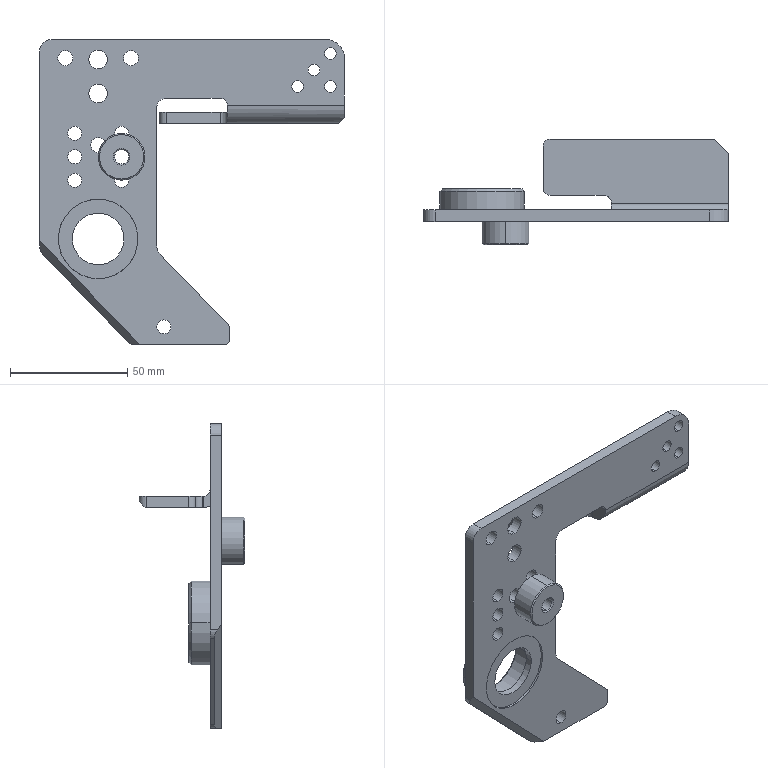Part | STEP file | Symmetry BALANCER 01 | 3 solids | 101 faces | box 130 x 45 x 130 mm | volume 53768 mm3 | cylinder 60 | plane 31 | cone 8 | torus 2 | commonest cylinder face diameters 6 x21 5 x8 6.4 x6 8.05 x4 10 x4 34 x4